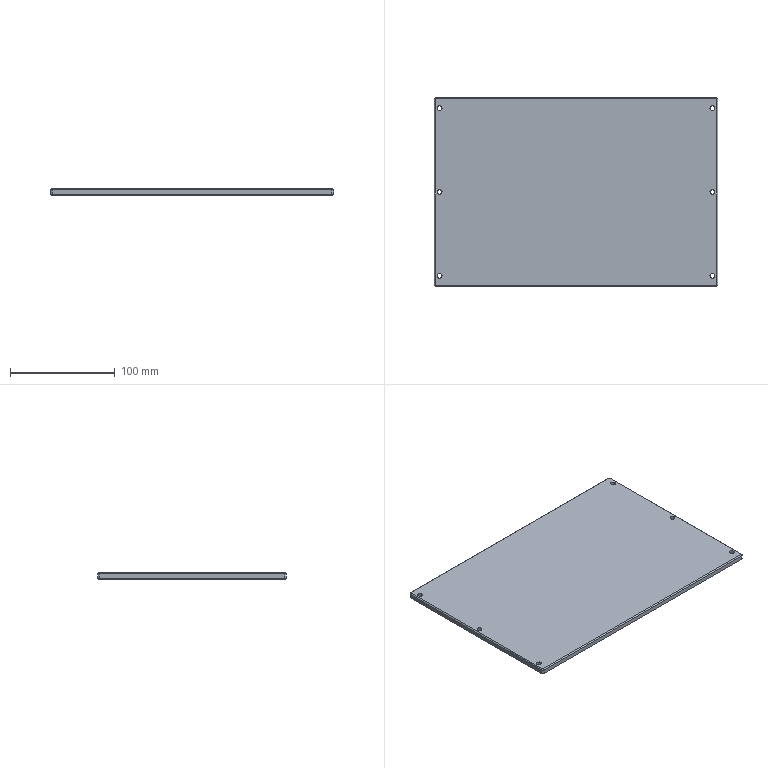Part | STEP file | 01-15 cover plate | 1 solid | 38 faces | box 270 x 180 x 6 mm | volume 290112 mm3 | cylinder 16 | plane 14 | cone 8 | commonest cylinder face diameters 4.5 x12 4 x4
STEP:
#1=CARTESIAN_POINT('',(132.25,-80.,6.));
#2=VERTEX_POINT('',#1);
#3=CARTESIAN_POINT('',(127.75,-80.,6.));
#4=VERTEX_POINT('',#3);
#5=CARTESIAN_POINT('',(130.,-80.,6.));
#6=DIRECTION('',(0.,0.,-1.));
#7=DIRECTION('',(1.,0.,0.));
#8=AXIS2_PLACEMENT_3D('',#5,#6,#7);
#9=CIRCLE('',#8,2.25);
#10=EDGE_CURVE('',#2,#4,#9,.T.);
#11=ORIENTED_EDGE('',*,*,#10,.F.);
#12=CARTESIAN_POINT('',(132.25,-80.,0.));
#13=VERTEX_POINT('',#12);
#14=CARTESIAN_POINT('',(132.25,-80.,10.));
#15=DIRECTION('',(0.,0.,-1.));
#16=VECTOR('',#15,1000.);
#17=LINE('',#14,#16);
#18=EDGE_CURVE('',#2,#13,#17,.T.);
#19=ORIENTED_EDGE('',*,*,#18,.T.);
#20=CARTESIAN_POINT('',(127.75,-80.,0.));
#21=VERTEX_POINT('',#20);
#22=CARTESIAN_POINT('',(130.,-80.,0.));
#23=DIRECTION('',(0.,0.,1.));
#24=DIRECTION('',(1.,0.,0.));
#25=AXIS2_PLACEMENT_3D('',#22,#23,#24);
#26=CIRCLE('',#25,2.25);
#27=EDGE_CURVE('',#21,#13,#26,.T.);
#28=ORIENTED_EDGE('',*,*,#27,.F.);
#29=CARTESIAN_POINT('',(127.75,-80.,10.));
#30=DIRECTION('',(0.,0.,-1.));
#31=VECTOR('',#30,1000.);
#32=LINE('',#29,#31);
#33=EDGE_CURVE('',#4,#21,#32,.T.);
#34=ORIENTED_EDGE('',*,*,#33,.F.);
#35=EDGE_LOOP('',(#11,#19,#28,#34));
#36=FACE_OUTER_BOUND('',#35,.T.);
#37=CARTESIAN_POINT('',(130.,-80.,10.));
#38=DIRECTION('',(0.,0.,-1.));
#39=DIRECTION('',(-1.,0.,0.));
#40=AXIS2_PLACEMENT_3D('',#37,#38,#39);
#41=CYLINDRICAL_SURFACE('',#40,2.25);
#42=ADVANCED_FACE('',(#36),#41,.F.);
#43=CARTESIAN_POINT('',(132.25,0.,6.));
#44=VERTEX_POINT('',#43);
#45=CARTESIAN_POINT('',(127.75,0.,6.));
#46=VERTEX_POINT('',#45);
#47=CARTESIAN_POINT('',(130.,0.,6.));
#48=DIRECTION('',(0.,0.,-1.));
#49=DIRECTION('',(1.,0.,0.));
#50=AXIS2_PLACEMENT_3D('',#47,#48,#49);
#51=CIRCLE('',#50,2.25);
#52=EDGE_CURVE('',#44,#46,#51,.T.);
#53=ORIENTED_EDGE('',*,*,#52,.F.);
#54=CARTESIAN_POINT('',(132.25,0.,0.));
#55=VERTEX_POINT('',#54);
#56=CARTESIAN_POINT('',(132.25,0.,10.));
#57=DIRECTION('',(0.,0.,-1.));
#58=VECTOR('',#57,1000.);
#59=LINE('',#56,#58);
#60=EDGE_CURVE('',#44,#55,#59,.T.);
#61=ORIENTED_EDGE('',*,*,#60,.T.);
#62=CARTESIAN_POINT('',(127.75,0.,0.));
#63=VERTEX_POINT('',#62);
#64=CARTESIAN_POINT('',(130.,0.,0.));
#65=DIRECTION('',(0.,0.,1.));
#66=DIRECTION('',(1.,0.,0.));
#67=AXIS2_PLACEMENT_3D('',#64,#65,#66);
#68=CIRCLE('',#67,2.25);
#69=EDGE_CURVE('',#63,#55,#68,.T.);
#70=ORIENTED_EDGE('',*,*,#69,.F.);
#71=CARTESIAN_POINT('',(127.75,0.,10.));
#72=DIRECTION('',(0.,0.,-1.));
#73=VECTOR('',#72,1000.);
#74=LINE('',#71,#73);
#75=EDGE_CURVE('',#46,#63,#74,.T.);
#76=ORIENTED_EDGE('',*,*,#75,.F.);
#77=EDGE_LOOP('',(#53,#61,#70,#76));
#78=FACE_OUTER_BOUND('',#77,.T.);
#79=CARTESIAN_POINT('',(130.,0.,10.));
#80=DIRECTION('',(0.,0.,-1.));
#81=DIRECTION('',(-1.,0.,0.));
#82=AXIS2_PLACEMENT_3D('',#79,#80,#81);
#83=CYLINDRICAL_SURFACE('',#82,2.25);
#84=ADVANCED_FACE('',(#78),#83,.F.);
#85=CARTESIAN_POINT('',(132.25,80.,6.));
#86=VERTEX_POINT('',#85);
#87=CARTESIAN_POINT('',(127.75,80.,6.));
#88=VERTEX_POINT('',#87);
#89=CARTESIAN_POINT('',(130.,80.,6.));
#90=DIRECTION('',(0.,0.,-1.));
#91=DIRECTION('',(1.,0.,0.));
#92=AXIS2_PLACEMENT_3D('',#89,#90,#91);
#93=CIRCLE('',#92,2.25);
#94=EDGE_CURVE('',#86,#88,#93,.T.);
#95=ORIENTED_EDGE('',*,*,#94,.F.);
#96=CARTESIAN_POINT('',(132.25,80.,0.));
#97=VERTEX_POINT('',#96);
#98=CARTESIAN_POINT('',(132.25,80.,10.));
#99=DIRECTION('',(0.,0.,-1.));
#100=VECTOR('',#99,1000.);
#101=LINE('',#98,#100);
#102=EDGE_CURVE('',#86,#97,#101,.T.);
#103=ORIENTED_EDGE('',*,*,#102,.T.);
#104=CARTESIAN_POINT('',(127.75,80.,0.));
#105=VERTEX_POINT('',#104);
#106=CARTESIAN_POINT('',(130.,80.,0.));
#107=DIRECTION('',(0.,0.,1.));
#108=DIRECTION('',(1.,0.,0.));
#109=AXIS2_PLACEMENT_3D('',#106,#107,#108);
#110=CIRCLE('',#109,2.25);
#111=EDGE_CURVE('',#105,#97,#110,.T.);
#112=ORIENTED_EDGE('',*,*,#111,.F.);
#113=CARTESIAN_POINT('',(127.75,80.,10.));
#114=DIRECTION('',(0.,0.,-1.));
#115=VECTOR('',#114,1000.);
#116=LINE('',#113,#115);
#117=EDGE_CURVE('',#88,#105,#116,.T.);
#118=ORIENTED_EDGE('',*,*,#117,.F.);
#119=EDGE_LOOP('',(#95,#103,#112,#118));
#120=FACE_OUTER_BOUND('',#119,.T.);
#121=CARTESIAN_POINT('',(130.,80.,10.));
#122=DIRECTION('',(0.,0.,-1.));
#123=DIRECTION('',(-1.,0.,0.));
#124=AXIS2_PLACEMENT_3D('',#121,#122,#123);
#125=CYLINDRICAL_SURFACE('',#124,2.25);
#126=ADVANCED_FACE('',(#120),#125,.F.);
#127=CARTESIAN_POINT('',(-132.25,-80.,6.));
#128=VERTEX_POINT('',#127);
#129=CARTESIAN_POINT('',(-127.75,-80.,6.));
#130=VERTEX_POINT('',#129);
#131=CARTESIAN_POINT('',(-130.,-80.,6.));
#132=DIRECTION('',(0.,0.,1.));
#133=DIRECTION('',(1.,0.,0.));
#134=AXIS2_PLACEMENT_3D('',#131,#132,#133);
#135=CIRCLE('',#134,2.25);
#136=EDGE_CURVE('',#128,#130,#135,.T.);
#137=ORIENTED_EDGE('',*,*,#136,.T.);
#138=CARTESIAN_POINT('',(-127.75,-80.,0.));
#139=VERTEX_POINT('',#138);
#140=CARTESIAN_POINT('',(-127.75,-80.,10.));
#141=DIRECTION('',(0.,0.,-1.));
#142=VECTOR('',#141,1000.);
#143=LINE('',#140,#142);
#144=EDGE_CURVE('',#130,#139,#143,.T.);
#145=ORIENTED_EDGE('',*,*,#144,.T.);
#146=CARTESIAN_POINT('',(-132.25,-80.,0.));
#147=VERTEX_POINT('',#146);
#148=CARTESIAN_POINT('',(-130.,-80.,0.));
#149=DIRECTION('',(0.,0.,-1.));
#150=DIRECTION('',(-1.,0.,0.));
#151=AXIS2_PLACEMENT_3D('',#148,#149,#150);
#152=CIRCLE('',#151,2.25);
#153=EDGE_CURVE('',#139,#147,#152,.T.);
#154=ORIENTED_EDGE('',*,*,#153,.T.);
#155=CARTESIAN_POINT('',(-132.25,-80.,10.));
#156=DIRECTION('',(0.,0.,-1.));
#157=VECTOR('',#156,1000.);
#158=LINE('',#155,#157);
#159=EDGE_CURVE('',#128,#147,#158,.T.);
#160=ORIENTED_EDGE('',*,*,#159,.F.);
#161=EDGE_LOOP('',(#137,#145,#154,#160));
#162=FACE_OUTER_BOUND('',#161,.T.);
#163=CARTESIAN_POINT('',(-130.,-80.,10.));
#164=DIRECTION('',(0.,0.,-1.));
#165=DIRECTION('',(-1.,0.,0.));
#166=AXIS2_PLACEMENT_3D('',#163,#164,#165);
#167=CYLINDRICAL_SURFACE('',#166,2.25);
#168=ADVANCED_FACE('',(#162),#167,.F.);
#169=CARTESIAN_POINT('',(-132.25,0.,6.));
#170=VERTEX_POINT('',#169);
#171=CARTESIAN_POINT('',(-127.75,0.,6.));
#172=VERTEX_POINT('',#171);
#173=CARTESIAN_POINT('',(-130.,0.,6.));
#174=DIRECTION('',(0.,0.,1.));
#175=DIRECTION('',(1.,0.,0.));
#176=AXIS2_PLACEMENT_3D('',#173,#174,#175);
#177=CIRCLE('',#176,2.25);
#178=EDGE_CURVE('',#170,#172,#177,.T.);
#179=ORIENTED_EDGE('',*,*,#178,.T.);
#180=CARTESIAN_POINT('',(-127.75,0.,0.));
#181=VERTEX_POINT('',#180);
#182=CARTESIAN_POINT('',(-127.75,0.,10.));
#183=DIRECTION('',(0.,0.,-1.));
#184=VECTOR('',#183,1000.);
#185=LINE('',#182,#184);
#186=EDGE_CURVE('',#172,#181,#185,.T.);
#187=ORIENTED_EDGE('',*,*,#186,.T.);
#188=CARTESIAN_POINT('',(-132.25,0.,0.));
#189=VERTEX_POINT('',#188);
#190=CARTESIAN_POINT('',(-130.,0.,0.));
#191=DIRECTION('',(0.,0.,-1.));
#192=DIRECTION('',(-1.,0.,0.));
#193=AXIS2_PLACEMENT_3D('',#190,#191,#192);
#194=CIRCLE('',#193,2.25);
#195=EDGE_CURVE('',#181,#189,#194,.T.);
#196=ORIENTED_EDGE('',*,*,#195,.T.);
#197=CARTESIAN_POINT('',(-132.25,0.,10.));
#198=DIRECTION('',(0.,0.,-1.));
#199=VECTOR('',#198,1000.);
#200=LINE('',#197,#199);
#201=EDGE_CURVE('',#170,#189,#200,.T.);
#202=ORIENTED_EDGE('',*,*,#201,.F.);
#203=EDGE_LOOP('',(#179,#187,#196,#202));
#204=FACE_OUTER_BOUND('',#203,.T.);
#205=CARTESIAN_POINT('',(-130.,0.,10.));
#206=DIRECTION('',(0.,0.,-1.));
#207=DIRECTION('',(-1.,0.,0.));
#208=AXIS2_PLACEMENT_3D('',#205,#206,#207);
#209=CYLINDRICAL_SURFACE('',#208,2.25);
#210=ADVANCED_FACE('',(#204),#209,.F.);
#211=CARTESIAN_POINT('',(-132.25,80.,6.));
#212=VERTEX_POINT('',#211);
#213=CARTESIAN_POINT('',(-127.75,80.,6.));
#214=VERTEX_POINT('',#213);
#215=CARTESIAN_POINT('',(-130.,80.,6.));
#216=DIRECTION('',(0.,0.,1.));
#217=DIRECTION('',(1.,0.,0.));
#218=AXIS2_PLACEMENT_3D('',#215,#216,#217);
#219=CIRCLE('',#218,2.25);
#220=EDGE_CURVE('',#212,#214,#219,.T.);
#221=ORIENTED_EDGE('',*,*,#220,.T.);
#222=CARTESIAN_POINT('',(-127.75,80.,0.));
#223=VERTEX_POINT('',#222);
#224=CARTESIAN_POINT('',(-127.75,80.,10.));
#225=DIRECTION('',(0.,0.,-1.));
#226=VECTOR('',#225,1000.);
#227=LINE('',#224,#226);
#228=EDGE_CURVE('',#214,#223,#227,.T.);
#229=ORIENTED_EDGE('',*,*,#228,.T.);
#230=CARTESIAN_POINT('',(-132.25,80.,0.));
#231=VERTEX_POINT('',#230);
#232=CARTESIAN_POINT('',(-130.,80.,0.));
#233=DIRECTION('',(0.,0.,-1.));
#234=DIRECTION('',(-1.,0.,0.));
#235=AXIS2_PLACEMENT_3D('',#232,#233,#234);
#236=CIRCLE('',#235,2.25);
#237=EDGE_CURVE('',#223,#231,#236,.T.);
#238=ORIENTED_EDGE('',*,*,#237,.T.);
#239=CARTESIAN_POINT('',(-132.25,80.,10.));
#240=DIRECTION('',(0.,0.,-1.));
#241=VECTOR('',#240,1000.);
#242=LINE('',#239,#241);
#243=EDGE_CURVE('',#212,#231,#242,.T.);
#244=ORIENTED_EDGE('',*,*,#243,.F.);
#245=EDGE_LOOP('',(#221,#229,#238,#244));
#246=FACE_OUTER_BOUND('',#245,.T.);
#247=CARTESIAN_POINT('',(-130.,80.,10.));
#248=DIRECTION('',(0.,0.,-1.));
#249=DIRECTION('',(-1.,0.,0.));
#250=AXIS2_PLACEMENT_3D('',#247,#248,#249);
#251=CYLINDRICAL_SURFACE('',#250,2.25);
#252=ADVANCED_FACE('',(#246),#251,.F.);
#253=CARTESIAN_POINT('',(130.,0.,6.));
#254=DIRECTION('',(0.,0.,-1.));
#255=DIRECTION('',(1.,0.,0.));
#256=AXIS2_PLACEMENT_3D('',#253,#254,#255);
#257=CIRCLE('',#256,2.25);
#258=EDGE_CURVE('',#46,#44,#257,.T.);
#259=ORIENTED_EDGE('',*,*,#258,.T.);
#260=ORIENTED_EDGE('',*,*,#52,.T.);
#261=EDGE_LOOP('',(#259,#260));
#262=FACE_BOUND('',#261,.T.);
#263=ORIENTED_EDGE('',*,*,#136,.F.);
#264=CARTESIAN_POINT('',(-130.,-80.,6.));
#265=DIRECTION('',(0.,0.,1.));
#266=DIRECTION('',(1.,0.,0.));
#267=AXIS2_PLACEMENT_3D('',#264,#265,#266);
#268=CIRCLE('',#267,2.25);
#269=EDGE_CURVE('',#130,#128,#268,.T.);
#270=ORIENTED_EDGE('',*,*,#269,.F.);
#271=EDGE_LOOP('',(#263,#270));
#272=FACE_BOUND('',#271,.T.);
#273=CARTESIAN_POINT('',(-133.,89.,6.));
#274=VERTEX_POINT('',#273);
#275=CARTESIAN_POINT('',(-134.,88.,6.));
#276=VERTEX_POINT('',#275);
#277=CARTESIAN_POINT('',(-133.,88.,6.));
#278=DIRECTION('',(0.,0.,1.));
#279=DIRECTION('',(1.,0.,0.));
#280=AXIS2_PLACEMENT_3D('',#277,#278,#279);
#281=CIRCLE('',#280,1.);
#282=EDGE_CURVE('',#274,#276,#281,.T.);
#283=ORIENTED_EDGE('',*,*,#282,.T.);
#284=CARTESIAN_POINT('',(-134.,-88.,6.));
#285=VERTEX_POINT('',#284);
#286=CARTESIAN_POINT('',(-134.,-88.,6.));
#287=DIRECTION('',(0.,-1.,0.));
#288=VECTOR('',#287,1000.);
#289=LINE('',#286,#288);
#290=EDGE_CURVE('',#276,#285,#289,.T.);
#291=ORIENTED_EDGE('',*,*,#290,.T.);
#292=CARTESIAN_POINT('',(-133.,-89.,6.));
#293=VERTEX_POINT('',#292);
#294=CARTESIAN_POINT('',(-133.,-88.,6.));
#295=DIRECTION('',(0.,0.,1.));
#296=DIRECTION('',(1.,0.,0.));
#297=AXIS2_PLACEMENT_3D('',#294,#295,#296);
#298=CIRCLE('',#297,1.);
#299=EDGE_CURVE('',#285,#293,#298,.T.);
#300=ORIENTED_EDGE('',*,*,#299,.T.);
#301=CARTESIAN_POINT('',(133.,-89.,6.));
#302=VERTEX_POINT('',#301);
#303=CARTESIAN_POINT('',(133.,-89.,6.));
#304=DIRECTION('',(1.,0.,0.));
#305=VECTOR('',#304,1000.);
#306=LINE('',#303,#305);
#307=EDGE_CURVE('',#293,#302,#306,.T.);
#308=ORIENTED_EDGE('',*,*,#307,.T.);
#309=CARTESIAN_POINT('',(134.,-88.,6.));
#310=VERTEX_POINT('',#309);
#311=CARTESIAN_POINT('',(133.,-88.,6.));
#312=DIRECTION('',(0.,0.,1.));
#313=DIRECTION('',(1.,0.,0.));
#314=AXIS2_PLACEMENT_3D('',#311,#312,#313);
#315=CIRCLE('',#314,1.);
#316=EDGE_CURVE('',#302,#310,#315,.T.);
#317=ORIENTED_EDGE('',*,*,#316,.T.);
#318=CARTESIAN_POINT('',(134.,88.,6.));
#319=VERTEX_POINT('',#318);
#320=CARTESIAN_POINT('',(134.,88.,6.));
#321=DIRECTION('',(0.,1.,0.));
#322=VECTOR('',#321,1000.);
#323=LINE('',#320,#322);
#324=EDGE_CURVE('',#310,#319,#323,.T.);
#325=ORIENTED_EDGE('',*,*,#324,.T.);
#326=CARTESIAN_POINT('',(133.,89.,6.));
#327=VERTEX_POINT('',#326);
#328=CARTESIAN_POINT('',(133.,88.,6.));
#329=DIRECTION('',(0.,0.,1.));
#330=DIRECTION('',(1.,0.,0.));
#331=AXIS2_PLACEMENT_3D('',#328,#329,#330);
#332=CIRCLE('',#331,1.);
#333=EDGE_CURVE('',#319,#327,#332,.T.);
#334=ORIENTED_EDGE('',*,*,#333,.T.);
#335=CARTESIAN_POINT('',(-133.,89.,6.));
#336=DIRECTION('',(-1.,0.,0.));
#337=VECTOR('',#336,1000.);
#338=LINE('',#335,#337);
#339=EDGE_CURVE('',#327,#274,#338,.T.);
#340=ORIENTED_EDGE('',*,*,#339,.T.);
#341=EDGE_LOOP('',(#283,#291,#300,#308,#317,#325,#334,#340));
#342=FACE_OUTER_BOUND('',#341,.T.);
#343=ORIENTED_EDGE('',*,*,#220,.F.);
#344=CARTESIAN_POINT('',(-130.,80.,6.));
#345=DIRECTION('',(0.,0.,1.));
#346=DIRECTION('',(1.,0.,0.));
#347=AXIS2_PLACEMENT_3D('',#344,#345,#346);
#348=CIRCLE('',#347,2.25);
#349=EDGE_CURVE('',#214,#212,#348,.T.);
#350=ORIENTED_EDGE('',*,*,#349,.F.);
#351=EDGE_LOOP('',(#343,#350));
#352=FACE_BOUND('',#351,.T.);
#353=ORIENTED_EDGE('',*,*,#178,.F.);
#354=CARTESIAN_POINT('',(-130.,0.,6.));
#355=DIRECTION('',(0.,0.,1.));
#356=DIRECTION('',(1.,0.,0.));
#357=AXIS2_PLACEMENT_3D('',#354,#355,#356);
#358=CIRCLE('',#357,2.25);
#359=EDGE_CURVE('',#172,#170,#358,.T.);
#360=ORIENTED_EDGE('',*,*,#359,.F.);
#361=EDGE_LOOP('',(#353,#360));
#362=FACE_BOUND('',#361,.T.);
#363=CARTESIAN_POINT('',(130.,80.,6.));
#364=DIRECTION('',(0.,0.,-1.));
#365=DIRECTION('',(1.,0.,0.));
#366=AXIS2_PLACEMENT_3D('',#363,#364,#365);
#367=CIRCLE('',#366,2.25);
#368=EDGE_CURVE('',#88,#86,#367,.T.);
#369=ORIENTED_EDGE('',*,*,#368,.T.);
#370=ORIENTED_EDGE('',*,*,#94,.T.);
#371=EDGE_LOOP('',(#369,#370));
#372=FACE_BOUND('',#371,.T.);
#373=CARTESIAN_POINT('',(130.,-80.,6.));
#374=DIRECTION('',(0.,0.,-1.));
#375=DIRECTION('',(1.,0.,0.));
#376=AXIS2_PLACEMENT_3D('',#373,#374,#375);
#377=CIRCLE('',#376,2.25);
#378=EDGE_CURVE('',#4,#2,#377,.T.);
#379=ORIENTED_EDGE('',*,*,#378,.T.);
#380=ORIENTED_EDGE('',*,*,#10,.T.);
#381=EDGE_LOOP('',(#379,#380));
#382=FACE_BOUND('',#381,.T.);
#383=CARTESIAN_POINT('',(135.,-90.,6.));
#384=DIRECTION('',(0.,0.,1.));
#385=DIRECTION('',(1.,0.,0.));
#386=AXIS2_PLACEMENT_3D('',#383,#384,#385);
#387=PLANE('',#386);
#388=ADVANCED_FACE('',(#262,#272,#342,#352,#362,#372,#382),#387,.T.);
#389=ORIENTED_EDGE('',*,*,#69,.T.);
#390=CARTESIAN_POINT('',(130.,0.,0.));
#391=DIRECTION('',(0.,0.,1.));
#392=DIRECTION('',(1.,0.,0.));
#393=AXIS2_PLACEMENT_3D('',#390,#391,#392);
#394=CIRCLE('',#393,2.25);
#395=EDGE_CURVE('',#55,#63,#394,.T.);
#396=ORIENTED_EDGE('',*,*,#395,.T.);
#397=EDGE_LOOP('',(#389,#396));
#398=FACE_BOUND('',#397,.T.);
#399=CARTESIAN_POINT('',(-130.,-80.,0.));
#400=DIRECTION('',(0.,0.,-1.));
#401=DIRECTION('',(-1.,0.,0.));
#402=AXIS2_PLACEMENT_3D('',#399,#400,#401);
#403=CIRCLE('',#402,2.25);
#404=EDGE_CURVE('',#147,#139,#403,.T.);
#405=ORIENTED_EDGE('',*,*,#404,.F.);
#406=ORIENTED_EDGE('',*,*,#153,.F.);
#407=EDGE_LOOP('',(#405,#406));
#408=FACE_BOUND('',#407,.T.);
#409=CARTESIAN_POINT('',(-133.,-89.,0.));
#410=VERTEX_POINT('',#409);
#411=CARTESIAN_POINT('',(-134.,-88.,0.));
#412=VERTEX_POINT('',#411);
#413=CARTESIAN_POINT('',(-133.,-88.,0.));
#414=DIRECTION('',(0.,0.,-1.));
#415=DIRECTION('',(1.,0.,0.));
#416=AXIS2_PLACEMENT_3D('',#413,#414,#415);
#417=CIRCLE('',#416,1.);
#418=EDGE_CURVE('',#410,#412,#417,.T.);
#419=ORIENTED_EDGE('',*,*,#418,.T.);
#420=CARTESIAN_POINT('',(-134.,88.,0.));
#421=VERTEX_POINT('',#420);
#422=CARTESIAN_POINT('',(-134.,-90.,0.));
#423=DIRECTION('',(0.,1.,0.));
#424=VECTOR('',#423,1000.);
#425=LINE('',#422,#424);
#426=EDGE_CURVE('',#412,#421,#425,.T.);
#427=ORIENTED_EDGE('',*,*,#426,.T.);
#428=CARTESIAN_POINT('',(-133.,89.,0.));
#429=VERTEX_POINT('',#428);
#430=CARTESIAN_POINT('',(-133.,88.,0.));
#431=DIRECTION('',(0.,0.,-1.));
#432=DIRECTION('',(1.,0.,0.));
#433=AXIS2_PLACEMENT_3D('',#430,#431,#432);
#434=CIRCLE('',#433,1.);
#435=EDGE_CURVE('',#421,#429,#434,.T.);
#436=ORIENTED_EDGE('',*,*,#435,.T.);
#437=CARTESIAN_POINT('',(133.,89.,0.));
#438=VERTEX_POINT('',#437);
#439=CARTESIAN_POINT('',(135.,89.,0.));
#440=DIRECTION('',(1.,0.,0.));
#441=VECTOR('',#440,1000.);
#442=LINE('',#439,#441);
#443=EDGE_CURVE('',#429,#438,#442,.T.);
#444=ORIENTED_EDGE('',*,*,#443,.T.);
#445=CARTESIAN_POINT('',(134.,88.,0.));
#446=VERTEX_POINT('',#445);
#447=CARTESIAN_POINT('',(133.,88.,0.));
#448=DIRECTION('',(0.,0.,-1.));
#449=DIRECTION('',(1.,0.,0.));
#450=AXIS2_PLACEMENT_3D('',#447,#448,#449);
#451=CIRCLE('',#450,1.);
#452=EDGE_CURVE('',#438,#446,#451,.T.);
#453=ORIENTED_EDGE('',*,*,#452,.T.);
#454=CARTESIAN_POINT('',(134.,-88.,0.));
#455=VERTEX_POINT('',#454);
#456=CARTESIAN_POINT('',(134.,-90.,0.));
#457=DIRECTION('',(0.,-1.,0.));
#458=VECTOR('',#457,1000.);
#459=LINE('',#456,#458);
#460=EDGE_CURVE('',#446,#455,#459,.T.);
#461=ORIENTED_EDGE('',*,*,#460,.T.);
#462=CARTESIAN_POINT('',(133.,-89.,0.));
#463=VERTEX_POINT('',#462);
#464=CARTESIAN_POINT('',(133.,-88.,0.));
#465=DIRECTION('',(0.,0.,-1.));
#466=DIRECTION('',(1.,0.,0.));
#467=AXIS2_PLACEMENT_3D('',#464,#465,#466);
#468=CIRCLE('',#467,1.);
#469=EDGE_CURVE('',#455,#463,#468,.T.);
#470=ORIENTED_EDGE('',*,*,#469,.T.);
#471=CARTESIAN_POINT('',(135.,-89.,0.));
#472=DIRECTION('',(-1.,0.,0.));
#473=VECTOR('',#472,1000.);
#474=LINE('',#471,#473);
#475=EDGE_CURVE('',#463,#410,#474,.T.);
#476=ORIENTED_EDGE('',*,*,#475,.T.);
#477=EDGE_LOOP('',(#419,#427,#436,#444,#453,#461,#470,#476));
#478=FACE_OUTER_BOUND('',#477,.T.);
#479=CARTESIAN_POINT('',(-130.,80.,0.));
#480=DIRECTION('',(0.,0.,-1.));
#481=DIRECTION('',(-1.,0.,0.));
#482=AXIS2_PLACEMENT_3D('',#479,#480,#481);
#483=CIRCLE('',#482,2.25);
#484=EDGE_CURVE('',#231,#223,#483,.T.);
#485=ORIENTED_EDGE('',*,*,#484,.F.);
#486=ORIENTED_EDGE('',*,*,#237,.F.);
#487=EDGE_LOOP('',(#485,#486));
#488=FACE_BOUND('',#487,.T.);
#489=CARTESIAN_POINT('',(-130.,0.,0.));
#490=DIRECTION('',(0.,0.,-1.));
#491=DIRECTION('',(-1.,0.,0.));
#492=AXIS2_PLACEMENT_3D('',#489,#490,#491);
#493=CIRCLE('',#492,2.25);
#494=EDGE_CURVE('',#189,#181,#493,.T.);
#495=ORIENTED_EDGE('',*,*,#494,.F.);
#496=ORIENTED_EDGE('',*,*,#195,.F.);
#497=EDGE_LOOP('',(#495,#496));
#498=FACE_BOUND('',#497,.T.);
#499=ORIENTED_EDGE('',*,*,#111,.T.);
#500=CARTESIAN_POINT('',(130.,80.,0.));
#501=DIRECTION('',(0.,0.,1.));
#502=DIRECTION('',(1.,0.,0.));
#503=AXIS2_PLACEMENT_3D('',#500,#501,#502);
#504=CIRCLE('',#503,2.25);
#505=EDGE_CURVE('',#97,#105,#504,.T.);
#506=ORIENTED_EDGE('',*,*,#505,.T.);
#507=EDGE_LOOP('',(#499,#506));
#508=FACE_BOUND('',#507,.T.);
#509=ORIENTED_EDGE('',*,*,#27,.T.);
#510=CARTESIAN_POINT('',(130.,-80.,0.));
#511=DIRECTION('',(0.,0.,1.));
#512=DIRECTION('',(1.,0.,0.));
#513=AXIS2_PLACEMENT_3D('',#510,#511,#512);
#514=CIRCLE('',#513,2.25);
#515=EDGE_CURVE('',#13,#21,#514,.T.);
#516=ORIENTED_EDGE('',*,*,#515,.T.);
#517=EDGE_LOOP('',(#509,#516));
#518=FACE_BOUND('',#517,.T.);
#519=CARTESIAN_POINT('',(135.,-90.,0.));
#520=DIRECTION('',(0.,0.,1.));
#521=DIRECTION('',(1.,0.,0.));
#522=AXIS2_PLACEMENT_3D('',#519,#520,#521);
#523=PLANE('',#522);
#524=ADVANCED_FACE('',(#398,#408,#478,#488,#498,#508,#518),#523,.F.);
#525=CARTESIAN_POINT('',(135.,-88.,5.));
#526=VERTEX_POINT('',#525);
#527=CARTESIAN_POINT('',(135.,-88.,1.));
#528=VERTEX_POINT('',#527);
#529=CARTESIAN_POINT('',(135.,-88.,6.));
#530=DIRECTION('',(0.,0.,-1.));
#531=VECTOR('',#530,1000.);
#532=LINE('',#529,#531);
#533=EDGE_CURVE('',#526,#528,#532,.T.);
#534=ORIENTED_EDGE('',*,*,#533,.T.);
#535=CARTESIAN_POINT('',(135.,88.,1.));
#536=VERTEX_POINT('',#535);
#537=CARTESIAN_POINT('',(135.,90.,1.));
#538=DIRECTION('',(0.,1.,0.));
#539=VECTOR('',#538,1000.);
#540=LINE('',#537,#539);
#541=EDGE_CURVE('',#528,#536,#540,.T.);
#542=ORIENTED_EDGE('',*,*,#541,.T.);
#543=CARTESIAN_POINT('',(135.,88.,5.));
#544=VERTEX_POINT('',#543);
#545=CARTESIAN_POINT('',(135.,88.,6.));
#546=DIRECTION('',(0.,0.,1.));
#547=VECTOR('',#546,1000.);
#548=LINE('',#545,#547);
#549=EDGE_CURVE('',#536,#544,#548,.T.);
#550=ORIENTED_EDGE('',*,*,#549,.T.);
#551=CARTESIAN_POINT('',(135.,-88.,5.));
#552=DIRECTION('',(0.,-1.,0.));
#553=VECTOR('',#552,1000.);
#554=LINE('',#551,#553);
#555=EDGE_CURVE('',#544,#526,#554,.T.);
#556=ORIENTED_EDGE('',*,*,#555,.T.);
#557=EDGE_LOOP('',(#534,#542,#550,#556));
#558=FACE_OUTER_BOUND('',#557,.T.);
#559=CARTESIAN_POINT('',(135.,90.,6.));
#560=DIRECTION('',(-1.,0.,0.));
#561=DIRECTION('',(0.,-1.,0.));
#562=AXIS2_PLACEMENT_3D('',#559,#560,#561);
#563=PLANE('',#562);
#564=ADVANCED_FACE('',(#558),#563,.F.);
#565=CARTESIAN_POINT('',(133.,90.,5.));
#566=VERTEX_POINT('',#565);
#567=CARTESIAN_POINT('',(133.,90.,1.));
#568=VERTEX_POINT('',#567);
#569=CARTESIAN_POINT('',(133.,90.,6.));
#570=DIRECTION('',(0.,0.,-1.));
#571=VECTOR('',#570,1000.);
#572=LINE('',#569,#571);
#573=EDGE_CURVE('',#566,#568,#572,.T.);
#574=ORIENTED_EDGE('',*,*,#573,.T.);
#575=CARTESIAN_POINT('',(-133.,90.,1.));
#576=VERTEX_POINT('',#575);
#577=CARTESIAN_POINT('',(-135.,90.,1.));
#578=DIRECTION('',(-1.,0.,0.));
#579=VECTOR('',#578,1000.);
#580=LINE('',#577,#579);
#581=EDGE_CURVE('',#568,#576,#580,.T.);
#582=ORIENTED_EDGE('',*,*,#581,.T.);
#583=CARTESIAN_POINT('',(-133.,90.,5.));
#584=VERTEX_POINT('',#583);
#585=CARTESIAN_POINT('',(-133.,90.,6.));
#586=DIRECTION('',(0.,0.,1.));
#587=VECTOR('',#586,1000.);
#588=LINE('',#585,#587);
#589=EDGE_CURVE('',#576,#584,#588,.T.);
#590=ORIENTED_EDGE('',*,*,#589,.T.);
#591=CARTESIAN_POINT('',(133.,90.,5.));
#592=DIRECTION('',(1.,0.,0.));
#593=VECTOR('',#592,1000.);
#594=LINE('',#591,#593);
#595=EDGE_CURVE('',#584,#566,#594,.T.);
#596=ORIENTED_EDGE('',*,*,#595,.T.);
#597=EDGE_LOOP('',(#574,#582,#590,#596));
#598=FACE_OUTER_BOUND('',#597,.T.);
#599=CARTESIAN_POINT('',(-135.,90.,6.));
#600=DIRECTION('',(0.,-1.,0.));
#601=DIRECTION('',(0.,0.,-1.));
#602=AXIS2_PLACEMENT_3D('',#599,#600,#601);
#603=PLANE('',#602);
#604=ADVANCED_FACE('',(#598),#603,.F.);
#605=CARTESIAN_POINT('',(-135.,88.,5.));
#606=VERTEX_POINT('',#605);
#607=CARTESIAN_POINT('',(-135.,88.,1.));
#608=VERTEX_POINT('',#607);
#609=CARTESIAN_POINT('',(-135.,88.,6.));
#610=DIRECTION('',(0.,0.,-1.));
#611=VECTOR('',#610,1000.);
#612=LINE('',#609,#611);
#613=EDGE_CURVE('',#606,#608,#612,.T.);
#614=ORIENTED_EDGE('',*,*,#613,.T.);
#615=CARTESIAN_POINT('',(-135.,-88.,1.));
#616=VERTEX_POINT('',#615);
#617=CARTESIAN_POINT('',(-135.,90.,1.));
#618=DIRECTION('',(0.,-1.,0.));
#619=VECTOR('',#618,1000.);
#620=LINE('',#617,#619);
#621=EDGE_CURVE('',#608,#616,#620,.T.);
#622=ORIENTED_EDGE('',*,*,#621,.T.);
#623=CARTESIAN_POINT('',(-135.,-88.,5.));
#624=VERTEX_POINT('',#623);
#625=CARTESIAN_POINT('',(-135.,-88.,6.));
#626=DIRECTION('',(0.,0.,1.));
#627=VECTOR('',#626,1000.);
#628=LINE('',#625,#627);
#629=EDGE_CURVE('',#616,#624,#628,.T.);
#630=ORIENTED_EDGE('',*,*,#629,.T.);
#631=CARTESIAN_POINT('',(-135.,88.,5.));
#632=DIRECTION('',(0.,1.,0.));
#633=VECTOR('',#632,1000.);
#634=LINE('',#631,#633);
#635=EDGE_CURVE('',#624,#606,#634,.T.);
#636=ORIENTED_EDGE('',*,*,#635,.T.);
#637=EDGE_LOOP('',(#614,#622,#630,#636));
#638=FACE_OUTER_BOUND('',#637,.T.);
#639=CARTESIAN_POINT('',(-135.,90.,6.));
#640=DIRECTION('',(1.,0.,0.));
#641=DIRECTION('',(0.,1.,0.));
#642=AXIS2_PLACEMENT_3D('',#639,#640,#641);
#643=PLANE('',#642);
#644=ADVANCED_FACE('',(#638),#643,.F.);
#645=CARTESIAN_POINT('',(-133.,-90.,5.));
#646=VERTEX_POINT('',#645);
#647=CARTESIAN_POINT('',(-133.,-90.,1.));
#648=VERTEX_POINT('',#647);
#649=CARTESIAN_POINT('',(-133.,-90.,6.));
#650=DIRECTION('',(0.,0.,-1.));
#651=VECTOR('',#650,1000.);
#652=LINE('',#649,#651);
#653=EDGE_CURVE('',#646,#648,#652,.T.);
#654=ORIENTED_EDGE('',*,*,#653,.T.);
#655=CARTESIAN_POINT('',(133.,-90.,1.));
#656=VERTEX_POINT('',#655);
#657=CARTESIAN_POINT('',(-135.,-90.,1.));
#658=DIRECTION('',(1.,0.,0.));
#659=VECTOR('',#658,1000.);
#660=LINE('',#657,#659);
#661=EDGE_CURVE('',#648,#656,#660,.T.);
#662=ORIENTED_EDGE('',*,*,#661,.T.);
#663=CARTESIAN_POINT('',(133.,-90.,5.));
#664=VERTEX_POINT('',#663);
#665=CARTESIAN_POINT('',(133.,-90.,6.));
#666=DIRECTION('',(0.,0.,1.));
#667=VECTOR('',#666,1000.);
#668=LINE('',#665,#667);
#669=EDGE_CURVE('',#656,#664,#668,.T.);
#670=ORIENTED_EDGE('',*,*,#669,.T.);
#671=CARTESIAN_POINT('',(-133.,-90.,5.));
#672=DIRECTION('',(-1.,0.,0.));
#673=VECTOR('',#672,1000.);
#674=LINE('',#671,#673);
#675=EDGE_CURVE('',#664,#646,#674,.T.);
#676=ORIENTED_EDGE('',*,*,#675,.T.);
#677=EDGE_LOOP('',(#654,#662,#670,#676));
#678=FACE_OUTER_BOUND('',#677,.T.);
#679=CARTESIAN_POINT('',(-135.,-90.,6.));
#680=DIRECTION('',(0.,1.,0.));
#681=DIRECTION('',(0.,0.,1.));
#682=AXIS2_PLACEMENT_3D('',#679,#680,#681);
#683=PLANE('',#682);
#684=ADVANCED_FACE('',(#678),#683,.F.);
#685=ORIENTED_EDGE('',*,*,#549,.F.);
#686=CARTESIAN_POINT('',(133.,88.,1.));
#687=DIRECTION('',(0.,0.,1.));
#688=DIRECTION('',(1.,0.,0.));
#689=AXIS2_PLACEMENT_3D('',#686,#687,#688);
#690=CIRCLE('',#689,2.);
#691=EDGE_CURVE('',#536,#568,#690,.T.);
#692=ORIENTED_EDGE('',*,*,#691,.T.);
#693=ORIENTED_EDGE('',*,*,#573,.F.);
#694=CARTESIAN_POINT('',(133.,88.,5.));
#695=DIRECTION('',(0.,0.,-1.));
#696=DIRECTION('',(1.,0.,0.));
#697=AXIS2_PLACEMENT_3D('',#694,#695,#696);
#698=CIRCLE('',#697,2.);
#699=EDGE_CURVE('',#566,#544,#698,.T.);
#700=ORIENTED_EDGE('',*,*,#699,.T.);
#701=EDGE_LOOP('',(#685,#692,#693,#700));
#702=FACE_OUTER_BOUND('',#701,.T.);
#703=CARTESIAN_POINT('',(133.,88.,6.));
#704=DIRECTION('',(0.,0.,-1.));
#705=DIRECTION('',(-1.,0.,0.));
#706=AXIS2_PLACEMENT_3D('',#703,#704,#705);
#707=CYLINDRICAL_SURFACE('',#706,2.);
#708=ADVANCED_FACE('',(#702),#707,.T.);
#709=ORIENTED_EDGE('',*,*,#669,.F.);
#710=CARTESIAN_POINT('',(133.,-88.,1.));
#711=DIRECTION('',(0.,0.,1.));
#712=DIRECTION('',(1.,0.,0.));
#713=AXIS2_PLACEMENT_3D('',#710,#711,#712);
#714=CIRCLE('',#713,2.);
#715=EDGE_CURVE('',#656,#528,#714,.T.);
#716=ORIENTED_EDGE('',*,*,#715,.T.);
#717=ORIENTED_EDGE('',*,*,#533,.F.);
#718=CARTESIAN_POINT('',(133.,-88.,5.));
#719=DIRECTION('',(0.,0.,-1.));
#720=DIRECTION('',(1.,0.,0.));
#721=AXIS2_PLACEMENT_3D('',#718,#719,#720);
#722=CIRCLE('',#721,2.);
#723=EDGE_CURVE('',#526,#664,#722,.T.);
#724=ORIENTED_EDGE('',*,*,#723,.T.);
#725=EDGE_LOOP('',(#709,#716,#717,#724));
#726=FACE_OUTER_BOUND('',#725,.T.);
#727=CARTESIAN_POINT('',(133.,-88.,6.));
#728=DIRECTION('',(0.,0.,-1.));
#729=DIRECTION('',(-1.,0.,0.));
#730=AXIS2_PLACEMENT_3D('',#727,#728,#729);
#731=CYLINDRICAL_SURFACE('',#730,2.);
#732=ADVANCED_FACE('',(#726),#731,.T.);
#733=ORIENTED_EDGE('',*,*,#589,.F.);
#734=CARTESIAN_POINT('',(-133.,88.,1.));
#735=DIRECTION('',(0.,0.,1.));
#736=DIRECTION('',(1.,0.,0.));
#737=AXIS2_PLACEMENT_3D('',#734,#735,#736);
#738=CIRCLE('',#737,2.);
#739=EDGE_CURVE('',#576,#608,#738,.T.);
#740=ORIENTED_EDGE('',*,*,#739,.T.);
#741=ORIENTED_EDGE('',*,*,#613,.F.);
#742=CARTESIAN_POINT('',(-133.,88.,5.));
#743=DIRECTION('',(0.,0.,-1.));
#744=DIRECTION('',(1.,0.,0.));
#745=AXIS2_PLACEMENT_3D('',#742,#743,#744);
#746=CIRCLE('',#745,2.);
#747=EDGE_CURVE('',#606,#584,#746,.T.);
#748=ORIENTED_EDGE('',*,*,#747,.T.);
#749=EDGE_LOOP('',(#733,#740,#741,#748));
#750=FACE_OUTER_BOUND('',#749,.T.);
#751=CARTESIAN_POINT('',(-133.,88.,6.));
#752=DIRECTION('',(0.,0.,-1.));
#753=DIRECTION('',(-1.,0.,0.));
#754=AXIS2_PLACEMENT_3D('',#751,#752,#753);
#755=CYLINDRICAL_SURFACE('',#754,2.);
#756=ADVANCED_FACE('',(#750),#755,.T.);
#757=ORIENTED_EDGE('',*,*,#629,.F.);
#758=CARTESIAN_POINT('',(-133.,-88.,1.));
#759=DIRECTION('',(0.,0.,1.));
#760=DIRECTION('',(1.,0.,0.));
#761=AXIS2_PLACEMENT_3D('',#758,#759,#760);
#762=CIRCLE('',#761,2.);
#763=EDGE_CURVE('',#616,#648,#762,.T.);
#764=ORIENTED_EDGE('',*,*,#763,.T.);
#765=ORIENTED_EDGE('',*,*,#653,.F.);
#766=CARTESIAN_POINT('',(-133.,-88.,5.));
#767=DIRECTION('',(0.,0.,-1.));
#768=DIRECTION('',(1.,0.,0.));
#769=AXIS2_PLACEMENT_3D('',#766,#767,#768);
#770=CIRCLE('',#769,2.);
#771=EDGE_CURVE('',#646,#624,#770,.T.);
#772=ORIENTED_EDGE('',*,*,#771,.T.);
#773=EDGE_LOOP('',(#757,#764,#765,#772));
#774=FACE_OUTER_BOUND('',#773,.T.);
#775=CARTESIAN_POINT('',(-133.,-88.,6.));
#776=DIRECTION('',(0.,0.,-1.));
#777=DIRECTION('',(-1.,0.,0.));
#778=AXIS2_PLACEMENT_3D('',#775,#776,#777);
#779=CYLINDRICAL_SURFACE('',#778,2.);
#780=ADVANCED_FACE('',(#774),#779,.T.);
#781=CARTESIAN_POINT('',(134.,-88.,0.));
#782=DIRECTION('',(0.7071,0.,0.7071));
#783=VECTOR('',#782,1000.);
#784=LINE('',#781,#783);
#785=EDGE_CURVE('',#455,#528,#784,.T.);
#786=ORIENTED_EDGE('',*,*,#785,.F.);
#787=ORIENTED_EDGE('',*,*,#460,.F.);
#788=CARTESIAN_POINT('',(135.,88.,1.));
#789=DIRECTION('',(-0.7071,0.,-0.7071));
#790=VECTOR('',#789,1000.);
#791=LINE('',#788,#790);
#792=EDGE_CURVE('',#536,#446,#791,.T.);
#793=ORIENTED_EDGE('',*,*,#792,.F.);
#794=ORIENTED_EDGE('',*,*,#541,.F.);
#795=EDGE_LOOP('',(#786,#787,#793,#794));
#796=FACE_OUTER_BOUND('',#795,.T.);
#797=CARTESIAN_POINT('',(135.,90.,1.));
#798=DIRECTION('',(-0.7071,0.,0.7071));
#799=DIRECTION('',(0.7071,0.,0.7071));
#800=AXIS2_PLACEMENT_3D('',#797,#798,#799);
#801=PLANE('',#800);
#802=ADVANCED_FACE('',(#796),#801,.F.);
#803=ORIENTED_EDGE('',*,*,#792,.T.);
#804=ORIENTED_EDGE('',*,*,#452,.F.);
#805=CARTESIAN_POINT('',(133.,90.,1.));
#806=DIRECTION('',(0.,-0.7071,-0.7071));
#807=VECTOR('',#806,1000.);
#808=LINE('',#805,#807);
#809=EDGE_CURVE('',#568,#438,#808,.T.);
#810=ORIENTED_EDGE('',*,*,#809,.F.);
#811=ORIENTED_EDGE('',*,*,#691,.F.);
#812=EDGE_LOOP('',(#803,#804,#810,#811));
#813=FACE_OUTER_BOUND('',#812,.T.);
#814=CARTESIAN_POINT('',(133.,88.,0.));
#815=DIRECTION('',(0.,0.,1.));
#816=DIRECTION('',(1.,0.,0.));
#817=AXIS2_PLACEMENT_3D('',#814,#815,#816);
#818=CONICAL_SURFACE('',#817,1.,0.7854);
#819=ADVANCED_FACE('',(#813),#818,.T.);
#820=ORIENTED_EDGE('',*,*,#785,.T.);
#821=ORIENTED_EDGE('',*,*,#715,.F.);
#822=CARTESIAN_POINT('',(133.,-89.,0.));
#823=DIRECTION('',(0.,-0.7071,0.7071));
#824=VECTOR('',#823,1000.);
#825=LINE('',#822,#824);
#826=EDGE_CURVE('',#463,#656,#825,.T.);
#827=ORIENTED_EDGE('',*,*,#826,.F.);
#828=ORIENTED_EDGE('',*,*,#469,.F.);
#829=EDGE_LOOP('',(#820,#821,#827,#828));
#830=FACE_OUTER_BOUND('',#829,.T.);
#831=CARTESIAN_POINT('',(133.,-88.,0.));
#832=DIRECTION('',(0.,0.,1.));
#833=DIRECTION('',(1.,0.,0.));
#834=AXIS2_PLACEMENT_3D('',#831,#832,#833);
#835=CONICAL_SURFACE('',#834,1.,0.7854);
#836=ADVANCED_FACE('',(#830),#835,.T.);
#837=ORIENTED_EDGE('',*,*,#809,.T.);
#838=ORIENTED_EDGE('',*,*,#443,.F.);
#839=CARTESIAN_POINT('',(-133.,90.,1.));
#840=DIRECTION('',(0.,-0.7071,-0.7071));
#841=VECTOR('',#840,1000.);
#842=LINE('',#839,#841);
#843=EDGE_CURVE('',#576,#429,#842,.T.);
#844=ORIENTED_EDGE('',*,*,#843,.F.);
#845=ORIENTED_EDGE('',*,*,#581,.F.);
#846=EDGE_LOOP('',(#837,#838,#844,#845));
#847=FACE_OUTER_BOUND('',#846,.T.);
#848=CARTESIAN_POINT('',(-135.,90.,1.));
#849=DIRECTION('',(0.,-0.7071,0.7071));
#850=DIRECTION('',(0.,-0.7071,-0.7071));
#851=AXIS2_PLACEMENT_3D('',#848,#849,#850);
#852=PLANE('',#851);
#853=ADVANCED_FACE('',(#847),#852,.F.);
#854=ORIENTED_EDGE('',*,*,#826,.T.);
#855=ORIENTED_EDGE('',*,*,#661,.F.);
#856=CARTESIAN_POINT('',(-133.,-89.,0.));
#857=DIRECTION('',(0.,-0.7071,0.7071));
#858=VECTOR('',#857,1000.);
#859=LINE('',#856,#858);
#860=EDGE_CURVE('',#410,#648,#859,.T.);
#861=ORIENTED_EDGE('',*,*,#860,.F.);
#862=ORIENTED_EDGE('',*,*,#475,.F.);
#863=EDGE_LOOP('',(#854,#855,#861,#862));
#864=FACE_OUTER_BOUND('',#863,.T.);
#865=CARTESIAN_POINT('',(-135.,-90.,1.));
#866=DIRECTION('',(0.,0.7071,0.7071));
#867=DIRECTION('',(0.,-0.7071,0.7071));
#868=AXIS2_PLACEMENT_3D('',#865,#866,#867);
#869=PLANE('',#868);
#870=ADVANCED_FACE('',(#864),#869,.F.);
#871=ORIENTED_EDGE('',*,*,#843,.T.);
#872=ORIENTED_EDGE('',*,*,#435,.F.);
#873=CARTESIAN_POINT('',(-135.,88.,1.));
#874=DIRECTION('',(0.7071,0.,-0.7071));
#875=VECTOR('',#874,1000.);
#876=LINE('',#873,#875);
#877=EDGE_CURVE('',#608,#421,#876,.T.);
#878=ORIENTED_EDGE('',*,*,#877,.F.);
#879=ORIENTED_EDGE('',*,*,#739,.F.);
#880=EDGE_LOOP('',(#871,#872,#878,#879));
#881=FACE_OUTER_BOUND('',#880,.T.);
#882=CARTESIAN_POINT('',(-133.,88.,0.));
#883=DIRECTION('',(0.,0.,1.));
#884=DIRECTION('',(1.,0.,0.));
#885=AXIS2_PLACEMENT_3D('',#882,#883,#884);
#886=CONICAL_SURFACE('',#885,1.,0.7854);
#887=ADVANCED_FACE('',(#881),#886,.T.);
#888=ORIENTED_EDGE('',*,*,#860,.T.);
#889=ORIENTED_EDGE('',*,*,#763,.F.);
#890=CARTESIAN_POINT('',(-134.,-88.,0.));
#891=DIRECTION('',(-0.7071,0.,0.7071));
#892=VECTOR('',#891,1000.);
#893=LINE('',#890,#892);
#894=EDGE_CURVE('',#412,#616,#893,.T.);
#895=ORIENTED_EDGE('',*,*,#894,.F.);
#896=ORIENTED_EDGE('',*,*,#418,.F.);
#897=EDGE_LOOP('',(#888,#889,#895,#896));
#898=FACE_OUTER_BOUND('',#897,.T.);
#899=CARTESIAN_POINT('',(-133.,-88.,0.));
#900=DIRECTION('',(0.,0.,1.));
#901=DIRECTION('',(1.,0.,0.));
#902=AXIS2_PLACEMENT_3D('',#899,#900,#901);
#903=CONICAL_SURFACE('',#902,1.,0.7854);
#904=ADVANCED_FACE('',(#898),#903,.T.);
#905=ORIENTED_EDGE('',*,*,#877,.T.);
#906=ORIENTED_EDGE('',*,*,#426,.F.);
#907=ORIENTED_EDGE('',*,*,#894,.T.);
#908=ORIENTED_EDGE('',*,*,#621,.F.);
#909=EDGE_LOOP('',(#905,#906,#907,#908));
#910=FACE_OUTER_BOUND('',#909,.T.);
#911=CARTESIAN_POINT('',(-135.,90.,1.));
#912=DIRECTION('',(0.7071,0.,0.7071));
#913=DIRECTION('',(0.7071,0.,-0.7071));
#914=AXIS2_PLACEMENT_3D('',#911,#912,#913);
#915=PLANE('',#914);
#916=ADVANCED_FACE('',(#910),#915,.F.);
#917=CARTESIAN_POINT('',(135.,-88.,5.));
#918=DIRECTION('',(-0.7071,0.,0.7071));
#919=VECTOR('',#918,1000.);
#920=LINE('',#917,#919);
#921=EDGE_CURVE('',#526,#310,#920,.T.);
#922=ORIENTED_EDGE('',*,*,#921,.F.);
#923=ORIENTED_EDGE('',*,*,#555,.F.);
#924=CARTESIAN_POINT('',(134.,88.,6.));
#925=DIRECTION('',(0.7071,0.,-0.7071));
#926=VECTOR('',#925,1000.);
#927=LINE('',#924,#926);
#928=EDGE_CURVE('',#319,#544,#927,.T.);
#929=ORIENTED_EDGE('',*,*,#928,.F.);
#930=ORIENTED_EDGE('',*,*,#324,.F.);
#931=EDGE_LOOP('',(#922,#923,#929,#930));
#932=FACE_OUTER_BOUND('',#931,.T.);
#933=CARTESIAN_POINT('',(134.,-90.,6.));
#934=DIRECTION('',(0.7071,0.,0.7071));
#935=DIRECTION('',(0.7071,0.,-0.7071));
#936=AXIS2_PLACEMENT_3D('',#933,#934,#935);
#937=PLANE('',#936);
#938=ADVANCED_FACE('',(#932),#937,.T.);
#939=ORIENTED_EDGE('',*,*,#928,.T.);
#940=ORIENTED_EDGE('',*,*,#699,.F.);
#941=CARTESIAN_POINT('',(133.,89.,6.));
#942=DIRECTION('',(0.,0.7071,-0.7071));
#943=VECTOR('',#942,1000.);
#944=LINE('',#941,#943);
#945=EDGE_CURVE('',#327,#566,#944,.T.);
#946=ORIENTED_EDGE('',*,*,#945,.F.);
#947=ORIENTED_EDGE('',*,*,#333,.F.);
#948=EDGE_LOOP('',(#939,#940,#946,#947));
#949=FACE_OUTER_BOUND('',#948,.T.);
#950=CARTESIAN_POINT('',(133.,88.,6.));
#951=DIRECTION('',(0.,0.,-1.));
#952=DIRECTION('',(-1.,0.,0.));
#953=AXIS2_PLACEMENT_3D('',#950,#951,#952);
#954=CONICAL_SURFACE('',#953,1.,0.7854);
#955=ADVANCED_FACE('',(#949),#954,.T.);
#956=ORIENTED_EDGE('',*,*,#921,.T.);
#957=ORIENTED_EDGE('',*,*,#316,.F.);
#958=CARTESIAN_POINT('',(133.,-90.,5.));
#959=DIRECTION('',(0.,0.7071,0.7071));
#960=VECTOR('',#959,1000.);
#961=LINE('',#958,#960);
#962=EDGE_CURVE('',#664,#302,#961,.T.);
#963=ORIENTED_EDGE('',*,*,#962,.F.);
#964=ORIENTED_EDGE('',*,*,#723,.F.);
#965=EDGE_LOOP('',(#956,#957,#963,#964));
#966=FACE_OUTER_BOUND('',#965,.T.);
#967=CARTESIAN_POINT('',(133.,-88.,6.));
#968=DIRECTION('',(0.,0.,-1.));
#969=DIRECTION('',(-1.,0.,0.));
#970=AXIS2_PLACEMENT_3D('',#967,#968,#969);
#971=CONICAL_SURFACE('',#970,1.,0.7854);
#972=ADVANCED_FACE('',(#966),#971,.T.);
#973=ORIENTED_EDGE('',*,*,#945,.T.);
#974=ORIENTED_EDGE('',*,*,#595,.F.);
#975=CARTESIAN_POINT('',(-133.,89.,6.));
#976=DIRECTION('',(0.,0.7071,-0.7071));
#977=VECTOR('',#976,1000.);
#978=LINE('',#975,#977);
#979=EDGE_CURVE('',#274,#584,#978,.T.);
#980=ORIENTED_EDGE('',*,*,#979,.F.);
#981=ORIENTED_EDGE('',*,*,#339,.F.);
#982=EDGE_LOOP('',(#973,#974,#980,#981));
#983=FACE_OUTER_BOUND('',#982,.T.);
#984=CARTESIAN_POINT('',(135.,89.,6.));
#985=DIRECTION('',(0.,0.7071,0.7071));
#986=DIRECTION('',(0.,-0.7071,0.7071));
#987=AXIS2_PLACEMENT_3D('',#984,#985,#986);
#988=PLANE('',#987);
#989=ADVANCED_FACE('',(#983),#988,.T.);
#990=ORIENTED_EDGE('',*,*,#962,.T.);
#991=ORIENTED_EDGE('',*,*,#307,.F.);
#992=CARTESIAN_POINT('',(-133.,-90.,5.));
#993=DIRECTION('',(0.,0.7071,0.7071));
#994=VECTOR('',#993,1000.);
#995=LINE('',#992,#994);
#996=EDGE_CURVE('',#646,#293,#995,.T.);
#997=ORIENTED_EDGE('',*,*,#996,.F.);
#998=ORIENTED_EDGE('',*,*,#675,.F.);
#999=EDGE_LOOP('',(#990,#991,#997,#998));
#1000=FACE_OUTER_BOUND('',#999,.T.);
#1001=CARTESIAN_POINT('',(135.,-89.,6.));
#1002=DIRECTION('',(0.,-0.7071,0.7071));
#1003=DIRECTION('',(0.,-0.7071,-0.7071));
#1004=AXIS2_PLACEMENT_3D('',#1001,#1002,#1003);
#1005=PLANE('',#1004);
#1006=ADVANCED_FACE('',(#1000),#1005,.T.);
#1007=ORIENTED_EDGE('',*,*,#979,.T.);
#1008=ORIENTED_EDGE('',*,*,#747,.F.);
#1009=CARTESIAN_POINT('',(-134.,88.,6.));
#1010=DIRECTION('',(-0.7071,0.,-0.7071));
#1011=VECTOR('',#1010,1000.);
#1012=LINE('',#1009,#1011);
#1013=EDGE_CURVE('',#276,#606,#1012,.T.);
#1014=ORIENTED_EDGE('',*,*,#1013,.F.);
#1015=ORIENTED_EDGE('',*,*,#282,.F.);
#1016=EDGE_LOOP('',(#1007,#1008,#1014,#1015));
#1017=FACE_OUTER_BOUND('',#1016,.T.);
#1018=CARTESIAN_POINT('',(-133.,88.,6.));
#1019=DIRECTION('',(0.,0.,-1.));
#1020=DIRECTION('',(-1.,0.,0.));
#1021=AXIS2_PLACEMENT_3D('',#1018,#1019,#1020);
#1022=CONICAL_SURFACE('',#1021,1.,0.7854);
#1023=ADVANCED_FACE('',(#1017),#1022,.T.);
#1024=ORIENTED_EDGE('',*,*,#996,.T.);
#1025=ORIENTED_EDGE('',*,*,#299,.F.);
#1026=CARTESIAN_POINT('',(-135.,-88.,5.));
#1027=DIRECTION('',(0.7071,0.,0.7071));
#1028=VECTOR('',#1027,1000.);
#1029=LINE('',#1026,#1028);
#1030=EDGE_CURVE('',#624,#285,#1029,.T.);
#1031=ORIENTED_EDGE('',*,*,#1030,.F.);
#1032=ORIENTED_EDGE('',*,*,#771,.F.);
#1033=EDGE_LOOP('',(#1024,#1025,#1031,#1032));
#1034=FACE_OUTER_BOUND('',#1033,.T.);
#1035=CARTESIAN_POINT('',(-133.,-88.,6.));
#1036=DIRECTION('',(0.,0.,-1.));
#1037=DIRECTION('',(-1.,0.,0.));
#1038=AXIS2_PLACEMENT_3D('',#1035,#1036,#1037);
#1039=CONICAL_SURFACE('',#1038,1.,0.7854);
#1040=ADVANCED_FACE('',(#1034),#1039,.T.);
#1041=ORIENTED_EDGE('',*,*,#1013,.T.);
#1042=ORIENTED_EDGE('',*,*,#635,.F.);
#1043=ORIENTED_EDGE('',*,*,#1030,.T.);
#1044=ORIENTED_EDGE('',*,*,#290,.F.);
#1045=EDGE_LOOP('',(#1041,#1042,#1043,#1044));
#1046=FACE_OUTER_BOUND('',#1045,.T.);
#1047=CARTESIAN_POINT('',(-134.,-90.,6.));
#1048=DIRECTION('',(-0.7071,0.,0.7071));
#1049=DIRECTION('',(0.7071,0.,0.7071));
#1050=AXIS2_PLACEMENT_3D('',#1047,#1048,#1049);
#1051=PLANE('',#1050);
#1052=ADVANCED_FACE('',(#1046),#1051,.T.);
#1053=ORIENTED_EDGE('',*,*,#228,.F.);
#1054=ORIENTED_EDGE('',*,*,#349,.T.);
#1055=ORIENTED_EDGE('',*,*,#243,.T.);
#1056=ORIENTED_EDGE('',*,*,#484,.T.);
#1057=EDGE_LOOP('',(#1053,#1054,#1055,#1056));
#1058=FACE_OUTER_BOUND('',#1057,.T.);
#1059=CARTESIAN_POINT('',(-130.,80.,10.));
#1060=DIRECTION('',(0.,0.,-1.));
#1061=DIRECTION('',(-1.,0.,0.));
#1062=AXIS2_PLACEMENT_3D('',#1059,#1060,#1061);
#1063=CYLINDRICAL_SURFACE('',#1062,2.25);
#1064=ADVANCED_FACE('',(#1058),#1063,.F.);
#1065=ORIENTED_EDGE('',*,*,#186,.F.);
#1066=ORIENTED_EDGE('',*,*,#359,.T.);
#1067=ORIENTED_EDGE('',*,*,#201,.T.);
#1068=ORIENTED_EDGE('',*,*,#494,.T.);
#1069=EDGE_LOOP('',(#1065,#1066,#1067,#1068));
#1070=FACE_OUTER_BOUND('',#1069,.T.);
#1071=CARTESIAN_POINT('',(-130.,0.,10.));
#1072=DIRECTION('',(0.,0.,-1.));
#1073=DIRECTION('',(-1.,0.,0.));
#1074=AXIS2_PLACEMENT_3D('',#1071,#1072,#1073);
#1075=CYLINDRICAL_SURFACE('',#1074,2.25);
#1076=ADVANCED_FACE('',(#1070),#1075,.F.);
#1077=ORIENTED_EDGE('',*,*,#144,.F.);
#1078=ORIENTED_EDGE('',*,*,#269,.T.);
#1079=ORIENTED_EDGE('',*,*,#159,.T.);
#1080=ORIENTED_EDGE('',*,*,#404,.T.);
#1081=EDGE_LOOP('',(#1077,#1078,#1079,#1080));
#1082=FACE_OUTER_BOUND('',#1081,.T.);
#1083=CARTESIAN_POINT('',(-130.,-80.,10.));
#1084=DIRECTION('',(0.,0.,-1.));
#1085=DIRECTION('',(-1.,0.,0.));
#1086=AXIS2_PLACEMENT_3D('',#1083,#1084,#1085);
#1087=CYLINDRICAL_SURFACE('',#1086,2.25);
#1088=ADVANCED_FACE('',(#1082),#1087,.F.);
#1089=ORIENTED_EDGE('',*,*,#102,.F.);
#1090=ORIENTED_EDGE('',*,*,#368,.F.);
#1091=ORIENTED_EDGE('',*,*,#117,.T.);
#1092=ORIENTED_EDGE('',*,*,#505,.F.);
#1093=EDGE_LOOP('',(#1089,#1090,#1091,#1092));
#1094=FACE_OUTER_BOUND('',#1093,.T.);
#1095=CARTESIAN_POINT('',(130.,80.,10.));
#1096=DIRECTION('',(0.,0.,-1.));
#1097=DIRECTION('',(-1.,0.,0.));
#1098=AXIS2_PLACEMENT_3D('',#1095,#1096,#1097);
#1099=CYLINDRICAL_SURFACE('',#1098,2.25);
#1100=ADVANCED_FACE('',(#1094),#1099,.F.);
#1101=ORIENTED_EDGE('',*,*,#60,.F.);
#1102=ORIENTED_EDGE('',*,*,#258,.F.);
#1103=ORIENTED_EDGE('',*,*,#75,.T.);
#1104=ORIENTED_EDGE('',*,*,#395,.F.);
#1105=EDGE_LOOP('',(#1101,#1102,#1103,#1104));
#1106=FACE_OUTER_BOUND('',#1105,.T.);
#1107=CARTESIAN_POINT('',(130.,0.,10.));
#1108=DIRECTION('',(0.,0.,-1.));
#1109=DIRECTION('',(-1.,0.,0.));
#1110=AXIS2_PLACEMENT_3D('',#1107,#1108,#1109);
#1111=CYLINDRICAL_SURFACE('',#1110,2.25);
#1112=ADVANCED_FACE('',(#1106),#1111,.F.);
#1113=ORIENTED_EDGE('',*,*,#18,.F.);
#1114=ORIENTED_EDGE('',*,*,#378,.F.);
#1115=ORIENTED_EDGE('',*,*,#33,.T.);
#1116=ORIENTED_EDGE('',*,*,#515,.F.);
#1117=EDGE_LOOP('',(#1113,#1114,#1115,#1116));
#1118=FACE_OUTER_BOUND('',#1117,.T.);
#1119=CARTESIAN_POINT('',(130.,-80.,10.));
#1120=DIRECTION('',(0.,0.,-1.));
#1121=DIRECTION('',(-1.,0.,0.));
#1122=AXIS2_PLACEMENT_3D('',#1119,#1120,#1121);
#1123=CYLINDRICAL_SURFACE('',#1122,2.25);
#1124=ADVANCED_FACE('',(#1118),#1123,.F.);
#1125=CLOSED_SHELL('',(#42,#84,#126,#168,#210,#252,#388,#524,#564,#604,#644,#684,#708,#732,#756,#780,#802,#819,#836,#853,#870,#887,#904,#916,#938,#955,#972,#989,#1006,#1023,#1040,#1052,#1064,#1076,#1088,#1100,#1112,#1124));
#1126=MANIFOLD_SOLID_BREP('',#1125);
#1127=CARTESIAN_POINT('',(0.,0.,0.));
#1128=DIRECTION('',(0.,0.,1.));
#1129=DIRECTION('',(1.,0.,0.));
#1130=AXIS2_PLACEMENT_3D('',#1127,#1128,#1129);
#1131=(LENGTH_UNIT()NAMED_UNIT(*)SI_UNIT(.MILLI.,.METRE.));
#1132=UNCERTAINTY_MEASURE_WITH_UNIT(LENGTH_MEASURE(0.00001),#1131,'','');
#1133=(NAMED_UNIT(*)PLANE_ANGLE_UNIT()SI_UNIT($,.RADIAN.));
#1134=(NAMED_UNIT(*)SI_UNIT($,.STERADIAN.)SOLID_ANGLE_UNIT());
#1135=(GEOMETRIC_REPRESENTATION_CONTEXT(3)GLOBAL_UNCERTAINTY_ASSIGNED_CONTEXT((#1132))GLOBAL_UNIT_ASSIGNED_CONTEXT((#1131,#1133,#1134))REPRESENTATION_CONTEXT('',''));
#1136=ADVANCED_BREP_SHAPE_REPRESENTATION('',(#1126,#1130),#1135);